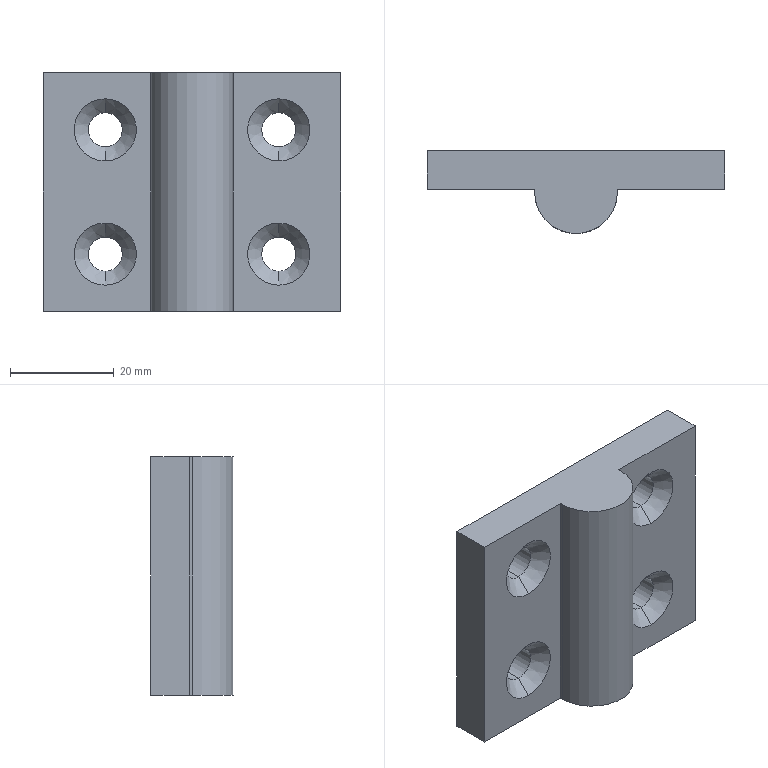Part | SolidWorks | features BaseBody 1 | 1 solid | 26 faces | box 57.5 x 16 x 46 mm | volume 23419 mm3 | cylinder 11 | cone 8 | plane 7 | commonest cylinder face diameters 6.6 x8 16 x3
STEP:
#1=CARTESIAN_POINT('',(-16.75,8.,-15.3));
#2=VERTEX_POINT('',#1);
#3=CARTESIAN_POINT('',(-16.75,8.,-8.7));
#4=VERTEX_POINT('',#3);
#5=CARTESIAN_POINT('',(-16.75,8.,-12.));
#6=DIRECTION('',(0.,1.,0.));
#7=DIRECTION('',(0.,0.,-1.));
#8=AXIS2_PLACEMENT_3D('',#5,#6,#7);
#9=CIRCLE('',#8,3.3);
#10=EDGE_CURVE('',#2,#4,#9,.T.);
#11=ORIENTED_EDGE('',*,*,#10,.T.);
#12=CARTESIAN_POINT('',(-16.75,3.2,-8.7));
#13=VERTEX_POINT('',#12);
#14=CARTESIAN_POINT('',(-16.75,0.5,-8.7));
#15=DIRECTION('',(0.,-1.,0.));
#16=VECTOR('',#15,1000.);
#17=LINE('',#14,#16);
#18=EDGE_CURVE('',#4,#13,#17,.T.);
#19=ORIENTED_EDGE('',*,*,#18,.T.);
#20=CARTESIAN_POINT('',(-16.75,3.2,-15.3));
#21=VERTEX_POINT('',#20);
#22=CARTESIAN_POINT('',(-16.75,3.2,-12.));
#23=DIRECTION('',(0.,1.,0.));
#24=DIRECTION('',(0.,0.,-1.));
#25=AXIS2_PLACEMENT_3D('',#22,#23,#24);
#26=CIRCLE('',#25,3.3);
#27=EDGE_CURVE('',#21,#13,#26,.T.);
#28=ORIENTED_EDGE('',*,*,#27,.F.);
#29=CARTESIAN_POINT('',(-16.75,0.5,-15.3));
#30=DIRECTION('',(0.,-1.,0.));
#31=VECTOR('',#30,1000.);
#32=LINE('',#29,#31);
#33=EDGE_CURVE('',#2,#21,#32,.T.);
#34=ORIENTED_EDGE('',*,*,#33,.F.);
#35=EDGE_LOOP('',(#11,#19,#28,#34));
#36=FACE_OUTER_BOUND('',#35,.T.);
#37=CARTESIAN_POINT('',(-16.75,0.5,-12.));
#38=DIRECTION('',(0.,-1.,0.));
#39=DIRECTION('',(0.,0.,-1.));
#40=AXIS2_PLACEMENT_3D('',#37,#38,#39);
#41=CYLINDRICAL_SURFACE('',#40,3.3);
#42=ADVANCED_FACE('',(#36),#41,.F.);
#43=CARTESIAN_POINT('',(16.75,8.,-15.3));
#44=VERTEX_POINT('',#43);
#45=CARTESIAN_POINT('',(16.75,8.,-8.7));
#46=VERTEX_POINT('',#45);
#47=CARTESIAN_POINT('',(16.75,8.,-12.));
#48=DIRECTION('',(0.,1.,0.));
#49=DIRECTION('',(0.,0.,-1.));
#50=AXIS2_PLACEMENT_3D('',#47,#48,#49);
#51=CIRCLE('',#50,3.3);
#52=EDGE_CURVE('',#44,#46,#51,.T.);
#53=ORIENTED_EDGE('',*,*,#52,.T.);
#54=CARTESIAN_POINT('',(16.75,3.2,-8.7));
#55=VERTEX_POINT('',#54);
#56=CARTESIAN_POINT('',(16.75,0.5,-8.7));
#57=DIRECTION('',(0.,-1.,0.));
#58=VECTOR('',#57,1000.);
#59=LINE('',#56,#58);
#60=EDGE_CURVE('',#46,#55,#59,.T.);
#61=ORIENTED_EDGE('',*,*,#60,.T.);
#62=CARTESIAN_POINT('',(16.75,3.2,-15.3));
#63=VERTEX_POINT('',#62);
#64=CARTESIAN_POINT('',(16.75,3.2,-12.));
#65=DIRECTION('',(0.,1.,0.));
#66=DIRECTION('',(0.,0.,-1.));
#67=AXIS2_PLACEMENT_3D('',#64,#65,#66);
#68=CIRCLE('',#67,3.3);
#69=EDGE_CURVE('',#63,#55,#68,.T.);
#70=ORIENTED_EDGE('',*,*,#69,.F.);
#71=CARTESIAN_POINT('',(16.75,0.5,-15.3));
#72=DIRECTION('',(0.,-1.,0.));
#73=VECTOR('',#72,1000.);
#74=LINE('',#71,#73);
#75=EDGE_CURVE('',#44,#63,#74,.T.);
#76=ORIENTED_EDGE('',*,*,#75,.F.);
#77=EDGE_LOOP('',(#53,#61,#70,#76));
#78=FACE_OUTER_BOUND('',#77,.T.);
#79=CARTESIAN_POINT('',(16.75,0.5,-12.));
#80=DIRECTION('',(0.,-1.,0.));
#81=DIRECTION('',(0.,0.,-1.));
#82=AXIS2_PLACEMENT_3D('',#79,#80,#81);
#83=CYLINDRICAL_SURFACE('',#82,3.3);
#84=ADVANCED_FACE('',(#78),#83,.F.);
#85=CARTESIAN_POINT('',(16.75,8.,8.7));
#86=VERTEX_POINT('',#85);
#87=CARTESIAN_POINT('',(16.75,8.,15.3));
#88=VERTEX_POINT('',#87);
#89=CARTESIAN_POINT('',(16.75,8.,12.));
#90=DIRECTION('',(0.,1.,0.));
#91=DIRECTION('',(0.,0.,-1.));
#92=AXIS2_PLACEMENT_3D('',#89,#90,#91);
#93=CIRCLE('',#92,3.3);
#94=EDGE_CURVE('',#86,#88,#93,.T.);
#95=ORIENTED_EDGE('',*,*,#94,.T.);
#96=CARTESIAN_POINT('',(16.75,3.2,15.3));
#97=VERTEX_POINT('',#96);
#98=CARTESIAN_POINT('',(16.75,0.5,15.3));
#99=DIRECTION('',(0.,-1.,0.));
#100=VECTOR('',#99,1000.);
#101=LINE('',#98,#100);
#102=EDGE_CURVE('',#88,#97,#101,.T.);
#103=ORIENTED_EDGE('',*,*,#102,.T.);
#104=CARTESIAN_POINT('',(16.75,3.2,8.7));
#105=VERTEX_POINT('',#104);
#106=CARTESIAN_POINT('',(16.75,3.2,12.));
#107=DIRECTION('',(0.,1.,0.));
#108=DIRECTION('',(0.,0.,-1.));
#109=AXIS2_PLACEMENT_3D('',#106,#107,#108);
#110=CIRCLE('',#109,3.3);
#111=EDGE_CURVE('',#105,#97,#110,.T.);
#112=ORIENTED_EDGE('',*,*,#111,.F.);
#113=CARTESIAN_POINT('',(16.75,0.5,8.7));
#114=DIRECTION('',(0.,-1.,0.));
#115=VECTOR('',#114,1000.);
#116=LINE('',#113,#115);
#117=EDGE_CURVE('',#86,#105,#116,.T.);
#118=ORIENTED_EDGE('',*,*,#117,.F.);
#119=EDGE_LOOP('',(#95,#103,#112,#118));
#120=FACE_OUTER_BOUND('',#119,.T.);
#121=CARTESIAN_POINT('',(16.75,0.5,12.));
#122=DIRECTION('',(0.,-1.,0.));
#123=DIRECTION('',(0.,0.,-1.));
#124=AXIS2_PLACEMENT_3D('',#121,#122,#123);
#125=CYLINDRICAL_SURFACE('',#124,3.3);
#126=ADVANCED_FACE('',(#120),#125,.F.);
#127=CARTESIAN_POINT('',(-16.75,8.,8.7));
#128=VERTEX_POINT('',#127);
#129=CARTESIAN_POINT('',(-16.75,8.,15.3));
#130=VERTEX_POINT('',#129);
#131=CARTESIAN_POINT('',(-16.75,8.,12.));
#132=DIRECTION('',(0.,1.,0.));
#133=DIRECTION('',(0.,0.,-1.));
#134=AXIS2_PLACEMENT_3D('',#131,#132,#133);
#135=CIRCLE('',#134,3.3);
#136=EDGE_CURVE('',#128,#130,#135,.T.);
#137=ORIENTED_EDGE('',*,*,#136,.T.);
#138=CARTESIAN_POINT('',(-16.75,3.2,15.3));
#139=VERTEX_POINT('',#138);
#140=CARTESIAN_POINT('',(-16.75,0.5,15.3));
#141=DIRECTION('',(0.,-1.,0.));
#142=VECTOR('',#141,1000.);
#143=LINE('',#140,#142);
#144=EDGE_CURVE('',#130,#139,#143,.T.);
#145=ORIENTED_EDGE('',*,*,#144,.T.);
#146=CARTESIAN_POINT('',(-16.75,3.2,8.7));
#147=VERTEX_POINT('',#146);
#148=CARTESIAN_POINT('',(-16.75,3.2,12.));
#149=DIRECTION('',(0.,1.,0.));
#150=DIRECTION('',(0.,0.,-1.));
#151=AXIS2_PLACEMENT_3D('',#148,#149,#150);
#152=CIRCLE('',#151,3.3);
#153=EDGE_CURVE('',#147,#139,#152,.T.);
#154=ORIENTED_EDGE('',*,*,#153,.F.);
#155=CARTESIAN_POINT('',(-16.75,0.5,8.7));
#156=DIRECTION('',(0.,-1.,0.));
#157=VECTOR('',#156,1000.);
#158=LINE('',#155,#157);
#159=EDGE_CURVE('',#128,#147,#158,.T.);
#160=ORIENTED_EDGE('',*,*,#159,.F.);
#161=EDGE_LOOP('',(#137,#145,#154,#160));
#162=FACE_OUTER_BOUND('',#161,.T.);
#163=CARTESIAN_POINT('',(-16.75,0.5,12.));
#164=DIRECTION('',(0.,-1.,0.));
#165=DIRECTION('',(0.,0.,-1.));
#166=AXIS2_PLACEMENT_3D('',#163,#164,#165);
#167=CYLINDRICAL_SURFACE('',#166,3.3);
#168=ADVANCED_FACE('',(#162),#167,.F.);
#169=CARTESIAN_POINT('',(8.,0.,23.));
#170=VERTEX_POINT('',#169);
#171=CARTESIAN_POINT('',(7.984,0.5,23.));
#172=VERTEX_POINT('',#171);
#173=CARTESIAN_POINT('',(0.,0.,23.));
#174=DIRECTION('',(0.,0.,1.));
#175=DIRECTION('',(-1.,0.,0.));
#176=AXIS2_PLACEMENT_3D('',#173,#174,#175);
#177=CIRCLE('',#176,8.);
#178=EDGE_CURVE('',#170,#172,#177,.T.);
#179=ORIENTED_EDGE('',*,*,#178,.F.);
#180=CARTESIAN_POINT('',(8.,0.,-23.));
#181=VERTEX_POINT('',#180);
#182=CARTESIAN_POINT('',(8.,0.,23.));
#183=DIRECTION('',(0.,0.,-1.));
#184=VECTOR('',#183,1000.);
#185=LINE('',#182,#184);
#186=EDGE_CURVE('',#170,#181,#185,.T.);
#187=ORIENTED_EDGE('',*,*,#186,.T.);
#188=CARTESIAN_POINT('',(7.984,0.5,-23.));
#189=VERTEX_POINT('',#188);
#190=CARTESIAN_POINT('',(0.,0.,-23.));
#191=DIRECTION('',(0.,0.,1.));
#192=DIRECTION('',(-1.,0.,0.));
#193=AXIS2_PLACEMENT_3D('',#190,#191,#192);
#194=CIRCLE('',#193,8.);
#195=EDGE_CURVE('',#181,#189,#194,.T.);
#196=ORIENTED_EDGE('',*,*,#195,.T.);
#197=CARTESIAN_POINT('',(7.984,0.5,23.));
#198=DIRECTION('',(0.,0.,1.));
#199=VECTOR('',#198,1000.);
#200=LINE('',#197,#199);
#201=EDGE_CURVE('',#189,#172,#200,.T.);
#202=ORIENTED_EDGE('',*,*,#201,.T.);
#203=EDGE_LOOP('',(#179,#187,#196,#202));
#204=FACE_OUTER_BOUND('',#203,.T.);
#205=CARTESIAN_POINT('',(0.,0.,23.));
#206=DIRECTION('',(0.,0.,-1.));
#207=DIRECTION('',(-1.,0.,0.));
#208=AXIS2_PLACEMENT_3D('',#205,#206,#207);
#209=CYLINDRICAL_SURFACE('',#208,8.);
#210=ADVANCED_FACE('',(#204),#209,.T.);
#211=ORIENTED_EDGE('',*,*,#186,.F.);
#212=CARTESIAN_POINT('',(-8.,0.,23.));
#213=VERTEX_POINT('',#212);
#214=CARTESIAN_POINT('',(0.,0.,23.));
#215=DIRECTION('',(0.,0.,1.));
#216=DIRECTION('',(-1.,0.,0.));
#217=AXIS2_PLACEMENT_3D('',#214,#215,#216);
#218=CIRCLE('',#217,8.);
#219=EDGE_CURVE('',#213,#170,#218,.T.);
#220=ORIENTED_EDGE('',*,*,#219,.F.);
#221=CARTESIAN_POINT('',(-8.,0.,-23.));
#222=VERTEX_POINT('',#221);
#223=CARTESIAN_POINT('',(-8.,0.,23.));
#224=DIRECTION('',(0.,0.,-1.));
#225=VECTOR('',#224,1000.);
#226=LINE('',#223,#225);
#227=EDGE_CURVE('',#213,#222,#226,.T.);
#228=ORIENTED_EDGE('',*,*,#227,.T.);
#229=CARTESIAN_POINT('',(0.,0.,-23.));
#230=DIRECTION('',(0.,0.,1.));
#231=DIRECTION('',(-1.,0.,0.));
#232=AXIS2_PLACEMENT_3D('',#229,#230,#231);
#233=CIRCLE('',#232,8.);
#234=EDGE_CURVE('',#222,#181,#233,.T.);
#235=ORIENTED_EDGE('',*,*,#234,.T.);
#236=EDGE_LOOP('',(#211,#220,#228,#235));
#237=FACE_OUTER_BOUND('',#236,.T.);
#238=CARTESIAN_POINT('',(0.,0.,23.));
#239=DIRECTION('',(0.,0.,-1.));
#240=DIRECTION('',(-1.,0.,0.));
#241=AXIS2_PLACEMENT_3D('',#238,#239,#240);
#242=CYLINDRICAL_SURFACE('',#241,8.);
#243=ADVANCED_FACE('',(#237),#242,.T.);
#244=ORIENTED_EDGE('',*,*,#27,.T.);
#245=CARTESIAN_POINT('',(-16.75,0.5,-6.));
#246=VERTEX_POINT('',#245);
#247=CARTESIAN_POINT('',(-16.75,0.5,-6.));
#248=DIRECTION('',(0.,-0.7071,0.7071));
#249=VECTOR('',#248,1000.);
#250=LINE('',#247,#249);
#251=EDGE_CURVE('',#13,#246,#250,.T.);
#252=ORIENTED_EDGE('',*,*,#251,.T.);
#253=CARTESIAN_POINT('',(-16.75,0.5,-18.));
#254=VERTEX_POINT('',#253);
#255=CARTESIAN_POINT('',(-16.75,0.5,-12.));
#256=DIRECTION('',(0.,-1.,0.));
#257=DIRECTION('',(0.,0.,-1.));
#258=AXIS2_PLACEMENT_3D('',#255,#256,#257);
#259=CIRCLE('',#258,6.);
#260=EDGE_CURVE('',#246,#254,#259,.T.);
#261=ORIENTED_EDGE('',*,*,#260,.T.);
#262=CARTESIAN_POINT('',(-16.75,0.5,-18.));
#263=DIRECTION('',(0.,-0.7071,-0.7071));
#264=VECTOR('',#263,1000.);
#265=LINE('',#262,#264);
#266=EDGE_CURVE('',#21,#254,#265,.T.);
#267=ORIENTED_EDGE('',*,*,#266,.F.);
#268=EDGE_LOOP('',(#244,#252,#261,#267));
#269=FACE_OUTER_BOUND('',#268,.T.);
#270=CARTESIAN_POINT('',(-16.75,0.5,-12.));
#271=DIRECTION('',(0.,-1.,0.));
#272=DIRECTION('',(0.,0.,-1.));
#273=AXIS2_PLACEMENT_3D('',#270,#271,#272);
#274=CONICAL_SURFACE('',#273,6.,0.7854);
#275=ADVANCED_FACE('',(#269),#274,.F.);
#276=ORIENTED_EDGE('',*,*,#69,.T.);
#277=CARTESIAN_POINT('',(16.75,0.5,-6.));
#278=VERTEX_POINT('',#277);
#279=CARTESIAN_POINT('',(16.75,0.5,-6.));
#280=DIRECTION('',(0.,-0.7071,0.7071));
#281=VECTOR('',#280,1000.);
#282=LINE('',#279,#281);
#283=EDGE_CURVE('',#55,#278,#282,.T.);
#284=ORIENTED_EDGE('',*,*,#283,.T.);
#285=CARTESIAN_POINT('',(16.75,0.5,-18.));
#286=VERTEX_POINT('',#285);
#287=CARTESIAN_POINT('',(16.75,0.5,-12.));
#288=DIRECTION('',(0.,-1.,0.));
#289=DIRECTION('',(0.,0.,-1.));
#290=AXIS2_PLACEMENT_3D('',#287,#288,#289);
#291=CIRCLE('',#290,6.);
#292=EDGE_CURVE('',#278,#286,#291,.T.);
#293=ORIENTED_EDGE('',*,*,#292,.T.);
#294=CARTESIAN_POINT('',(16.75,0.5,-18.));
#295=DIRECTION('',(0.,-0.7071,-0.7071));
#296=VECTOR('',#295,1000.);
#297=LINE('',#294,#296);
#298=EDGE_CURVE('',#63,#286,#297,.T.);
#299=ORIENTED_EDGE('',*,*,#298,.F.);
#300=EDGE_LOOP('',(#276,#284,#293,#299));
#301=FACE_OUTER_BOUND('',#300,.T.);
#302=CARTESIAN_POINT('',(16.75,0.5,-12.));
#303=DIRECTION('',(0.,-1.,0.));
#304=DIRECTION('',(0.,0.,-1.));
#305=AXIS2_PLACEMENT_3D('',#302,#303,#304);
#306=CONICAL_SURFACE('',#305,6.,0.7854);
#307=ADVANCED_FACE('',(#301),#306,.F.);
#308=ORIENTED_EDGE('',*,*,#111,.T.);
#309=CARTESIAN_POINT('',(16.75,0.5,18.));
#310=VERTEX_POINT('',#309);
#311=CARTESIAN_POINT('',(16.75,0.5,18.));
#312=DIRECTION('',(0.,-0.7071,0.7071));
#313=VECTOR('',#312,1000.);
#314=LINE('',#311,#313);
#315=EDGE_CURVE('',#97,#310,#314,.T.);
#316=ORIENTED_EDGE('',*,*,#315,.T.);
#317=CARTESIAN_POINT('',(16.75,0.5,6.));
#318=VERTEX_POINT('',#317);
#319=CARTESIAN_POINT('',(16.75,0.5,12.));
#320=DIRECTION('',(0.,-1.,0.));
#321=DIRECTION('',(0.,0.,-1.));
#322=AXIS2_PLACEMENT_3D('',#319,#320,#321);
#323=CIRCLE('',#322,6.);
#324=EDGE_CURVE('',#310,#318,#323,.T.);
#325=ORIENTED_EDGE('',*,*,#324,.T.);
#326=CARTESIAN_POINT('',(16.75,0.5,6.));
#327=DIRECTION('',(0.,-0.7071,-0.7071));
#328=VECTOR('',#327,1000.);
#329=LINE('',#326,#328);
#330=EDGE_CURVE('',#105,#318,#329,.T.);
#331=ORIENTED_EDGE('',*,*,#330,.F.);
#332=EDGE_LOOP('',(#308,#316,#325,#331));
#333=FACE_OUTER_BOUND('',#332,.T.);
#334=CARTESIAN_POINT('',(16.75,0.5,12.));
#335=DIRECTION('',(0.,-1.,0.));
#336=DIRECTION('',(0.,0.,-1.));
#337=AXIS2_PLACEMENT_3D('',#334,#335,#336);
#338=CONICAL_SURFACE('',#337,6.,0.7854);
#339=ADVANCED_FACE('',(#333),#338,.F.);
#340=ORIENTED_EDGE('',*,*,#153,.T.);
#341=CARTESIAN_POINT('',(-16.75,0.5,18.));
#342=VERTEX_POINT('',#341);
#343=CARTESIAN_POINT('',(-16.75,0.5,18.));
#344=DIRECTION('',(0.,-0.7071,0.7071));
#345=VECTOR('',#344,1000.);
#346=LINE('',#343,#345);
#347=EDGE_CURVE('',#139,#342,#346,.T.);
#348=ORIENTED_EDGE('',*,*,#347,.T.);
#349=CARTESIAN_POINT('',(-16.75,0.5,6.));
#350=VERTEX_POINT('',#349);
#351=CARTESIAN_POINT('',(-16.75,0.5,12.));
#352=DIRECTION('',(0.,-1.,0.));
#353=DIRECTION('',(0.,0.,-1.));
#354=AXIS2_PLACEMENT_3D('',#351,#352,#353);
#355=CIRCLE('',#354,6.);
#356=EDGE_CURVE('',#342,#350,#355,.T.);
#357=ORIENTED_EDGE('',*,*,#356,.T.);
#358=CARTESIAN_POINT('',(-16.75,0.5,6.));
#359=DIRECTION('',(0.,-0.7071,-0.7071));
#360=VECTOR('',#359,1000.);
#361=LINE('',#358,#360);
#362=EDGE_CURVE('',#147,#350,#361,.T.);
#363=ORIENTED_EDGE('',*,*,#362,.F.);
#364=EDGE_LOOP('',(#340,#348,#357,#363));
#365=FACE_OUTER_BOUND('',#364,.T.);
#366=CARTESIAN_POINT('',(-16.75,0.5,12.));
#367=DIRECTION('',(0.,-1.,0.));
#368=DIRECTION('',(0.,0.,-1.));
#369=AXIS2_PLACEMENT_3D('',#366,#367,#368);
#370=CONICAL_SURFACE('',#369,6.,0.7854);
#371=ADVANCED_FACE('',(#365),#370,.F.);
#372=CARTESIAN_POINT('',(-28.75,8.,23.));
#373=VERTEX_POINT('',#372);
#374=CARTESIAN_POINT('',(-28.75,8.,-23.));
#375=VERTEX_POINT('',#374);
#376=CARTESIAN_POINT('',(-28.75,8.,23.));
#377=DIRECTION('',(0.,0.,-1.));
#378=VECTOR('',#377,1000.);
#379=LINE('',#376,#378);
#380=EDGE_CURVE('',#373,#375,#379,.T.);
#381=ORIENTED_EDGE('',*,*,#380,.F.);
#382=CARTESIAN_POINT('',(28.75,8.,23.));
#383=VERTEX_POINT('',#382);
#384=CARTESIAN_POINT('',(-28.75,8.,23.));
#385=DIRECTION('',(-1.,0.,0.));
#386=VECTOR('',#385,1000.);
#387=LINE('',#384,#386);
#388=EDGE_CURVE('',#383,#373,#387,.T.);
#389=ORIENTED_EDGE('',*,*,#388,.F.);
#390=CARTESIAN_POINT('',(28.75,8.,-23.));
#391=VERTEX_POINT('',#390);
#392=CARTESIAN_POINT('',(28.75,8.,23.));
#393=DIRECTION('',(0.,0.,1.));
#394=VECTOR('',#393,1000.);
#395=LINE('',#392,#394);
#396=EDGE_CURVE('',#391,#383,#395,.T.);
#397=ORIENTED_EDGE('',*,*,#396,.F.);
#398=CARTESIAN_POINT('',(-28.75,8.,-23.));
#399=DIRECTION('',(1.,0.,0.));
#400=VECTOR('',#399,1000.);
#401=LINE('',#398,#400);
#402=EDGE_CURVE('',#375,#391,#401,.T.);
#403=ORIENTED_EDGE('',*,*,#402,.F.);
#404=EDGE_LOOP('',(#381,#389,#397,#403));
#405=FACE_OUTER_BOUND('',#404,.T.);
#406=ORIENTED_EDGE('',*,*,#10,.F.);
#407=CARTESIAN_POINT('',(-16.75,8.,-12.));
#408=DIRECTION('',(0.,1.,0.));
#409=DIRECTION('',(0.,0.,-1.));
#410=AXIS2_PLACEMENT_3D('',#407,#408,#409);
#411=CIRCLE('',#410,3.3);
#412=EDGE_CURVE('',#4,#2,#411,.T.);
#413=ORIENTED_EDGE('',*,*,#412,.F.);
#414=EDGE_LOOP('',(#406,#413));
#415=FACE_BOUND('',#414,.T.);
#416=ORIENTED_EDGE('',*,*,#52,.F.);
#417=CARTESIAN_POINT('',(16.75,8.,-12.));
#418=DIRECTION('',(0.,1.,0.));
#419=DIRECTION('',(0.,0.,-1.));
#420=AXIS2_PLACEMENT_3D('',#417,#418,#419);
#421=CIRCLE('',#420,3.3);
#422=EDGE_CURVE('',#46,#44,#421,.T.);
#423=ORIENTED_EDGE('',*,*,#422,.F.);
#424=EDGE_LOOP('',(#416,#423));
#425=FACE_BOUND('',#424,.T.);
#426=ORIENTED_EDGE('',*,*,#94,.F.);
#427=CARTESIAN_POINT('',(16.75,8.,12.));
#428=DIRECTION('',(0.,1.,0.));
#429=DIRECTION('',(0.,0.,-1.));
#430=AXIS2_PLACEMENT_3D('',#427,#428,#429);
#431=CIRCLE('',#430,3.3);
#432=EDGE_CURVE('',#88,#86,#431,.T.);
#433=ORIENTED_EDGE('',*,*,#432,.F.);
#434=EDGE_LOOP('',(#426,#433));
#435=FACE_BOUND('',#434,.T.);
#436=ORIENTED_EDGE('',*,*,#136,.F.);
#437=CARTESIAN_POINT('',(-16.75,8.,12.));
#438=DIRECTION('',(0.,1.,0.));
#439=DIRECTION('',(0.,0.,-1.));
#440=AXIS2_PLACEMENT_3D('',#437,#438,#439);
#441=CIRCLE('',#440,3.3);
#442=EDGE_CURVE('',#130,#128,#441,.T.);
#443=ORIENTED_EDGE('',*,*,#442,.F.);
#444=EDGE_LOOP('',(#436,#443));
#445=FACE_BOUND('',#444,.T.);
#446=CARTESIAN_POINT('',(-28.75,8.,23.));
#447=DIRECTION('',(0.,-1.,0.));
#448=DIRECTION('',(1.,0.,0.));
#449=AXIS2_PLACEMENT_3D('',#446,#447,#448);
#450=PLANE('',#449);
#451=ADVANCED_FACE('',(#405,#415,#425,#435,#445),#450,.F.);
#452=CARTESIAN_POINT('',(-28.75,0.5,-23.));
#453=VERTEX_POINT('',#452);
#454=CARTESIAN_POINT('',(-7.984,0.5,-23.));
#455=VERTEX_POINT('',#454);
#456=CARTESIAN_POINT('',(0.,0.5,-23.));
#457=DIRECTION('',(1.,0.,0.));
#458=VECTOR('',#457,1000.);
#459=LINE('',#456,#458);
#460=EDGE_CURVE('',#453,#455,#459,.T.);
#461=ORIENTED_EDGE('',*,*,#460,.F.);
#462=CARTESIAN_POINT('',(-28.75,0.,-23.));
#463=DIRECTION('',(0.,-1.,0.));
#464=VECTOR('',#463,1000.);
#465=LINE('',#462,#464);
#466=EDGE_CURVE('',#375,#453,#465,.T.);
#467=ORIENTED_EDGE('',*,*,#466,.F.);
#468=ORIENTED_EDGE('',*,*,#402,.T.);
#469=CARTESIAN_POINT('',(28.75,0.5,-23.));
#470=VERTEX_POINT('',#469);
#471=CARTESIAN_POINT('',(28.75,0.,-23.));
#472=DIRECTION('',(0.,1.,0.));
#473=VECTOR('',#472,1000.);
#474=LINE('',#471,#473);
#475=EDGE_CURVE('',#470,#391,#474,.T.);
#476=ORIENTED_EDGE('',*,*,#475,.F.);
#477=CARTESIAN_POINT('',(0.,0.5,-23.));
#478=DIRECTION('',(1.,0.,0.));
#479=VECTOR('',#478,1000.);
#480=LINE('',#477,#479);
#481=EDGE_CURVE('',#189,#470,#480,.T.);
#482=ORIENTED_EDGE('',*,*,#481,.F.);
#483=ORIENTED_EDGE('',*,*,#195,.F.);
#484=ORIENTED_EDGE('',*,*,#234,.F.);
#485=CARTESIAN_POINT('',(0.,0.,-23.));
#486=DIRECTION('',(0.,0.,1.));
#487=DIRECTION('',(-1.,0.,0.));
#488=AXIS2_PLACEMENT_3D('',#485,#486,#487);
#489=CIRCLE('',#488,8.);
#490=EDGE_CURVE('',#455,#222,#489,.T.);
#491=ORIENTED_EDGE('',*,*,#490,.F.);
#492=EDGE_LOOP('',(#461,#467,#468,#476,#482,#483,#484,#491));
#493=FACE_OUTER_BOUND('',#492,.T.);
#494=CARTESIAN_POINT('',(0.,0.,-23.));
#495=DIRECTION('',(0.,0.,1.));
#496=DIRECTION('',(1.,0.,0.));
#497=AXIS2_PLACEMENT_3D('',#494,#495,#496);
#498=PLANE('',#497);
#499=ADVANCED_FACE('',(#493),#498,.F.);
#500=CARTESIAN_POINT('',(-28.75,0.5,23.));
#501=VERTEX_POINT('',#500);
#502=CARTESIAN_POINT('',(-28.75,0.5,23.));
#503=DIRECTION('',(0.,0.,-1.));
#504=VECTOR('',#503,1000.);
#505=LINE('',#502,#504);
#506=EDGE_CURVE('',#501,#453,#505,.T.);
#507=ORIENTED_EDGE('',*,*,#506,.F.);
#508=CARTESIAN_POINT('',(-28.75,8.,23.));
#509=DIRECTION('',(0.,-1.,0.));
#510=VECTOR('',#509,1000.);
#511=LINE('',#508,#510);
#512=EDGE_CURVE('',#373,#501,#511,.T.);
#513=ORIENTED_EDGE('',*,*,#512,.F.);
#514=ORIENTED_EDGE('',*,*,#380,.T.);
#515=ORIENTED_EDGE('',*,*,#466,.T.);
#516=EDGE_LOOP('',(#507,#513,#514,#515));
#517=FACE_OUTER_BOUND('',#516,.T.);
#518=CARTESIAN_POINT('',(-28.75,8.,23.));
#519=DIRECTION('',(1.,0.,0.));
#520=DIRECTION('',(0.,0.,-1.));
#521=AXIS2_PLACEMENT_3D('',#518,#519,#520);
#522=PLANE('',#521);
#523=ADVANCED_FACE('',(#517),#522,.F.);
#524=ORIENTED_EDGE('',*,*,#512,.T.);
#525=CARTESIAN_POINT('',(-7.984,0.5,23.));
#526=VERTEX_POINT('',#525);
#527=CARTESIAN_POINT('',(0.,0.5,23.));
#528=DIRECTION('',(1.,0.,0.));
#529=VECTOR('',#528,1000.);
#530=LINE('',#527,#529);
#531=EDGE_CURVE('',#501,#526,#530,.T.);
#532=ORIENTED_EDGE('',*,*,#531,.T.);
#533=CARTESIAN_POINT('',(0.,0.,23.));
#534=DIRECTION('',(0.,0.,1.));
#535=DIRECTION('',(-1.,0.,0.));
#536=AXIS2_PLACEMENT_3D('',#533,#534,#535);
#537=CIRCLE('',#536,8.);
#538=EDGE_CURVE('',#526,#213,#537,.T.);
#539=ORIENTED_EDGE('',*,*,#538,.T.);
#540=ORIENTED_EDGE('',*,*,#219,.T.);
#541=ORIENTED_EDGE('',*,*,#178,.T.);
#542=CARTESIAN_POINT('',(28.75,0.5,23.));
#543=VERTEX_POINT('',#542);
#544=CARTESIAN_POINT('',(0.,0.5,23.));
#545=DIRECTION('',(1.,0.,0.));
#546=VECTOR('',#545,1000.);
#547=LINE('',#544,#546);
#548=EDGE_CURVE('',#172,#543,#547,.T.);
#549=ORIENTED_EDGE('',*,*,#548,.T.);
#550=CARTESIAN_POINT('',(28.75,0.,23.));
#551=DIRECTION('',(0.,1.,0.));
#552=VECTOR('',#551,1000.);
#553=LINE('',#550,#552);
#554=EDGE_CURVE('',#543,#383,#553,.T.);
#555=ORIENTED_EDGE('',*,*,#554,.T.);
#556=ORIENTED_EDGE('',*,*,#388,.T.);
#557=EDGE_LOOP('',(#524,#532,#539,#540,#541,#549,#555,#556));
#558=FACE_OUTER_BOUND('',#557,.T.);
#559=CARTESIAN_POINT('',(0.,0.,23.));
#560=DIRECTION('',(0.,0.,1.));
#561=DIRECTION('',(1.,0.,0.));
#562=AXIS2_PLACEMENT_3D('',#559,#560,#561);
#563=PLANE('',#562);
#564=ADVANCED_FACE('',(#558),#563,.T.);
#565=ORIENTED_EDGE('',*,*,#396,.T.);
#566=ORIENTED_EDGE('',*,*,#554,.F.);
#567=CARTESIAN_POINT('',(28.75,0.5,23.));
#568=DIRECTION('',(0.,0.,1.));
#569=VECTOR('',#568,1000.);
#570=LINE('',#567,#569);
#571=EDGE_CURVE('',#470,#543,#570,.T.);
#572=ORIENTED_EDGE('',*,*,#571,.F.);
#573=ORIENTED_EDGE('',*,*,#475,.T.);
#574=EDGE_LOOP('',(#565,#566,#572,#573));
#575=FACE_OUTER_BOUND('',#574,.T.);
#576=CARTESIAN_POINT('',(28.75,8.,23.));
#577=DIRECTION('',(-1.,0.,0.));
#578=DIRECTION('',(0.,0.,1.));
#579=AXIS2_PLACEMENT_3D('',#576,#577,#578);
#580=PLANE('',#579);
#581=ADVANCED_FACE('',(#575),#580,.F.);
#582=ORIENTED_EDGE('',*,*,#18,.F.);
#583=ORIENTED_EDGE('',*,*,#412,.T.);
#584=ORIENTED_EDGE('',*,*,#33,.T.);
#585=CARTESIAN_POINT('',(-16.75,3.2,-12.));
#586=DIRECTION('',(0.,1.,0.));
#587=DIRECTION('',(0.,0.,-1.));
#588=AXIS2_PLACEMENT_3D('',#585,#586,#587);
#589=CIRCLE('',#588,3.3);
#590=EDGE_CURVE('',#13,#21,#589,.T.);
#591=ORIENTED_EDGE('',*,*,#590,.F.);
#592=EDGE_LOOP('',(#582,#583,#584,#591));
#593=FACE_OUTER_BOUND('',#592,.T.);
#594=CARTESIAN_POINT('',(-16.75,0.5,-12.));
#595=DIRECTION('',(0.,-1.,0.));
#596=DIRECTION('',(0.,0.,-1.));
#597=AXIS2_PLACEMENT_3D('',#594,#595,#596);
#598=CYLINDRICAL_SURFACE('',#597,3.3);
#599=ADVANCED_FACE('',(#593),#598,.F.);
#600=ORIENTED_EDGE('',*,*,#60,.F.);
#601=ORIENTED_EDGE('',*,*,#422,.T.);
#602=ORIENTED_EDGE('',*,*,#75,.T.);
#603=CARTESIAN_POINT('',(16.75,3.2,-12.));
#604=DIRECTION('',(0.,1.,0.));
#605=DIRECTION('',(0.,0.,-1.));
#606=AXIS2_PLACEMENT_3D('',#603,#604,#605);
#607=CIRCLE('',#606,3.3);
#608=EDGE_CURVE('',#55,#63,#607,.T.);
#609=ORIENTED_EDGE('',*,*,#608,.F.);
#610=EDGE_LOOP('',(#600,#601,#602,#609));
#611=FACE_OUTER_BOUND('',#610,.T.);
#612=CARTESIAN_POINT('',(16.75,0.5,-12.));
#613=DIRECTION('',(0.,-1.,0.));
#614=DIRECTION('',(0.,0.,-1.));
#615=AXIS2_PLACEMENT_3D('',#612,#613,#614);
#616=CYLINDRICAL_SURFACE('',#615,3.3);
#617=ADVANCED_FACE('',(#611),#616,.F.);
#618=ORIENTED_EDGE('',*,*,#102,.F.);
#619=ORIENTED_EDGE('',*,*,#432,.T.);
#620=ORIENTED_EDGE('',*,*,#117,.T.);
#621=CARTESIAN_POINT('',(16.75,3.2,12.));
#622=DIRECTION('',(0.,1.,0.));
#623=DIRECTION('',(0.,0.,-1.));
#624=AXIS2_PLACEMENT_3D('',#621,#622,#623);
#625=CIRCLE('',#624,3.3);
#626=EDGE_CURVE('',#97,#105,#625,.T.);
#627=ORIENTED_EDGE('',*,*,#626,.F.);
#628=EDGE_LOOP('',(#618,#619,#620,#627));
#629=FACE_OUTER_BOUND('',#628,.T.);
#630=CARTESIAN_POINT('',(16.75,0.5,12.));
#631=DIRECTION('',(0.,-1.,0.));
#632=DIRECTION('',(0.,0.,-1.));
#633=AXIS2_PLACEMENT_3D('',#630,#631,#632);
#634=CYLINDRICAL_SURFACE('',#633,3.3);
#635=ADVANCED_FACE('',(#629),#634,.F.);
#636=ORIENTED_EDGE('',*,*,#144,.F.);
#637=ORIENTED_EDGE('',*,*,#442,.T.);
#638=ORIENTED_EDGE('',*,*,#159,.T.);
#639=CARTESIAN_POINT('',(-16.75,3.2,12.));
#640=DIRECTION('',(0.,1.,0.));
#641=DIRECTION('',(0.,0.,-1.));
#642=AXIS2_PLACEMENT_3D('',#639,#640,#641);
#643=CIRCLE('',#642,3.3);
#644=EDGE_CURVE('',#139,#147,#643,.T.);
#645=ORIENTED_EDGE('',*,*,#644,.F.);
#646=EDGE_LOOP('',(#636,#637,#638,#645));
#647=FACE_OUTER_BOUND('',#646,.T.);
#648=CARTESIAN_POINT('',(-16.75,0.5,12.));
#649=DIRECTION('',(0.,-1.,0.));
#650=DIRECTION('',(0.,0.,-1.));
#651=AXIS2_PLACEMENT_3D('',#648,#649,#650);
#652=CYLINDRICAL_SURFACE('',#651,3.3);
#653=ADVANCED_FACE('',(#647),#652,.F.);
#654=CARTESIAN_POINT('',(-7.984,0.5,23.));
#655=DIRECTION('',(0.,0.,-1.));
#656=VECTOR('',#655,1000.);
#657=LINE('',#654,#656);
#658=EDGE_CURVE('',#526,#455,#657,.T.);
#659=ORIENTED_EDGE('',*,*,#658,.F.);
#660=ORIENTED_EDGE('',*,*,#531,.F.);
#661=ORIENTED_EDGE('',*,*,#506,.T.);
#662=ORIENTED_EDGE('',*,*,#460,.T.);
#663=EDGE_LOOP('',(#659,#660,#661,#662));
#664=FACE_OUTER_BOUND('',#663,.T.);
#665=CARTESIAN_POINT('',(-16.75,0.5,-12.));
#666=DIRECTION('',(0.,-1.,0.));
#667=DIRECTION('',(0.,0.,-1.));
#668=AXIS2_PLACEMENT_3D('',#665,#666,#667);
#669=CIRCLE('',#668,6.);
#670=EDGE_CURVE('',#254,#246,#669,.T.);
#671=ORIENTED_EDGE('',*,*,#670,.F.);
#672=ORIENTED_EDGE('',*,*,#260,.F.);
#673=EDGE_LOOP('',(#671,#672));
#674=FACE_BOUND('',#673,.T.);
#675=CARTESIAN_POINT('',(-16.75,0.5,12.));
#676=DIRECTION('',(0.,-1.,0.));
#677=DIRECTION('',(0.,0.,-1.));
#678=AXIS2_PLACEMENT_3D('',#675,#676,#677);
#679=CIRCLE('',#678,6.);
#680=EDGE_CURVE('',#350,#342,#679,.T.);
#681=ORIENTED_EDGE('',*,*,#680,.F.);
#682=ORIENTED_EDGE('',*,*,#356,.F.);
#683=EDGE_LOOP('',(#681,#682));
#684=FACE_BOUND('',#683,.T.);
#685=CARTESIAN_POINT('',(-28.75,0.5,23.));
#686=DIRECTION('',(0.,1.,0.));
#687=DIRECTION('',(-1.,0.,0.));
#688=AXIS2_PLACEMENT_3D('',#685,#686,#687);
#689=PLANE('',#688);
#690=ADVANCED_FACE('',(#664,#674,#684),#689,.F.);
#691=ORIENTED_EDGE('',*,*,#571,.T.);
#692=ORIENTED_EDGE('',*,*,#548,.F.);
#693=ORIENTED_EDGE('',*,*,#201,.F.);
#694=ORIENTED_EDGE('',*,*,#481,.T.);
#695=EDGE_LOOP('',(#691,#692,#693,#694));
#696=FACE_OUTER_BOUND('',#695,.T.);
#697=CARTESIAN_POINT('',(16.75,0.5,-12.));
#698=DIRECTION('',(0.,-1.,0.));
#699=DIRECTION('',(0.,0.,-1.));
#700=AXIS2_PLACEMENT_3D('',#697,#698,#699);
#701=CIRCLE('',#700,6.);
#702=EDGE_CURVE('',#286,#278,#701,.T.);
#703=ORIENTED_EDGE('',*,*,#702,.F.);
#704=ORIENTED_EDGE('',*,*,#292,.F.);
#705=EDGE_LOOP('',(#703,#704));
#706=FACE_BOUND('',#705,.T.);
#707=CARTESIAN_POINT('',(16.75,0.5,12.));
#708=DIRECTION('',(0.,-1.,0.));
#709=DIRECTION('',(0.,0.,-1.));
#710=AXIS2_PLACEMENT_3D('',#707,#708,#709);
#711=CIRCLE('',#710,6.);
#712=EDGE_CURVE('',#318,#310,#711,.T.);
#713=ORIENTED_EDGE('',*,*,#712,.F.);
#714=ORIENTED_EDGE('',*,*,#324,.F.);
#715=EDGE_LOOP('',(#713,#714));
#716=FACE_BOUND('',#715,.T.);
#717=CARTESIAN_POINT('',(7.984,0.5,23.));
#718=DIRECTION('',(0.,1.,0.));
#719=DIRECTION('',(-1.,0.,0.));
#720=AXIS2_PLACEMENT_3D('',#717,#718,#719);
#721=PLANE('',#720);
#722=ADVANCED_FACE('',(#696,#706,#716),#721,.F.);
#723=ORIENTED_EDGE('',*,*,#227,.F.);
#724=ORIENTED_EDGE('',*,*,#538,.F.);
#725=ORIENTED_EDGE('',*,*,#658,.T.);
#726=ORIENTED_EDGE('',*,*,#490,.T.);
#727=EDGE_LOOP('',(#723,#724,#725,#726));
#728=FACE_OUTER_BOUND('',#727,.T.);
#729=CARTESIAN_POINT('',(0.,0.,23.));
#730=DIRECTION('',(0.,0.,-1.));
#731=DIRECTION('',(-1.,0.,0.));
#732=AXIS2_PLACEMENT_3D('',#729,#730,#731);
#733=CYLINDRICAL_SURFACE('',#732,8.);
#734=ADVANCED_FACE('',(#728),#733,.T.);
#735=ORIENTED_EDGE('',*,*,#251,.F.);
#736=ORIENTED_EDGE('',*,*,#590,.T.);
#737=ORIENTED_EDGE('',*,*,#266,.T.);
#738=ORIENTED_EDGE('',*,*,#670,.T.);
#739=EDGE_LOOP('',(#735,#736,#737,#738));
#740=FACE_OUTER_BOUND('',#739,.T.);
#741=CARTESIAN_POINT('',(-16.75,0.5,-12.));
#742=DIRECTION('',(0.,-1.,0.));
#743=DIRECTION('',(0.,0.,-1.));
#744=AXIS2_PLACEMENT_3D('',#741,#742,#743);
#745=CONICAL_SURFACE('',#744,6.,0.7854);
#746=ADVANCED_FACE('',(#740),#745,.F.);
#747=ORIENTED_EDGE('',*,*,#283,.F.);
#748=ORIENTED_EDGE('',*,*,#608,.T.);
#749=ORIENTED_EDGE('',*,*,#298,.T.);
#750=ORIENTED_EDGE('',*,*,#702,.T.);
#751=EDGE_LOOP('',(#747,#748,#749,#750));
#752=FACE_OUTER_BOUND('',#751,.T.);
#753=CARTESIAN_POINT('',(16.75,0.5,-12.));
#754=DIRECTION('',(0.,-1.,0.));
#755=DIRECTION('',(0.,0.,-1.));
#756=AXIS2_PLACEMENT_3D('',#753,#754,#755);
#757=CONICAL_SURFACE('',#756,6.,0.7854);
#758=ADVANCED_FACE('',(#752),#757,.F.);
#759=ORIENTED_EDGE('',*,*,#315,.F.);
#760=ORIENTED_EDGE('',*,*,#626,.T.);
#761=ORIENTED_EDGE('',*,*,#330,.T.);
#762=ORIENTED_EDGE('',*,*,#712,.T.);
#763=EDGE_LOOP('',(#759,#760,#761,#762));
#764=FACE_OUTER_BOUND('',#763,.T.);
#765=CARTESIAN_POINT('',(16.75,0.5,12.));
#766=DIRECTION('',(0.,-1.,0.));
#767=DIRECTION('',(0.,0.,-1.));
#768=AXIS2_PLACEMENT_3D('',#765,#766,#767);
#769=CONICAL_SURFACE('',#768,6.,0.7854);
#770=ADVANCED_FACE('',(#764),#769,.F.);
#771=ORIENTED_EDGE('',*,*,#347,.F.);
#772=ORIENTED_EDGE('',*,*,#644,.T.);
#773=ORIENTED_EDGE('',*,*,#362,.T.);
#774=ORIENTED_EDGE('',*,*,#680,.T.);
#775=EDGE_LOOP('',(#771,#772,#773,#774));
#776=FACE_OUTER_BOUND('',#775,.T.);
#777=CARTESIAN_POINT('',(-16.75,0.5,12.));
#778=DIRECTION('',(0.,-1.,0.));
#779=DIRECTION('',(0.,0.,-1.));
#780=AXIS2_PLACEMENT_3D('',#777,#778,#779);
#781=CONICAL_SURFACE('',#780,6.,0.7854);
#782=ADVANCED_FACE('',(#776),#781,.F.);
#783=CLOSED_SHELL('',(#42,#84,#126,#168,#210,#243,#275,#307,#339,#371,#451,#499,#523,#564,#581,#599,#617,#635,#653,#690,#722,#734,#746,#758,#770,#782));
#784=MANIFOLD_SOLID_BREP('',#783);
#785=CARTESIAN_POINT('',(0.,0.,0.));
#786=DIRECTION('',(0.,0.,1.));
#787=DIRECTION('',(1.,0.,0.));
#788=AXIS2_PLACEMENT_3D('',#785,#786,#787);
#789=(LENGTH_UNIT()NAMED_UNIT(*)SI_UNIT(.MILLI.,.METRE.));
#790=UNCERTAINTY_MEASURE_WITH_UNIT(LENGTH_MEASURE(0.00001),#789,'','');
#791=(NAMED_UNIT(*)PLANE_ANGLE_UNIT()SI_UNIT($,.RADIAN.));
#792=(NAMED_UNIT(*)SI_UNIT($,.STERADIAN.)SOLID_ANGLE_UNIT());
#793=(GEOMETRIC_REPRESENTATION_CONTEXT(3)GLOBAL_UNCERTAINTY_ASSIGNED_CONTEXT((#790))GLOBAL_UNIT_ASSIGNED_CONTEXT((#789,#791,#792))REPRESENTATION_CONTEXT('',''));
#794=ADVANCED_BREP_SHAPE_REPRESENTATION('',(#784,#788),#793);